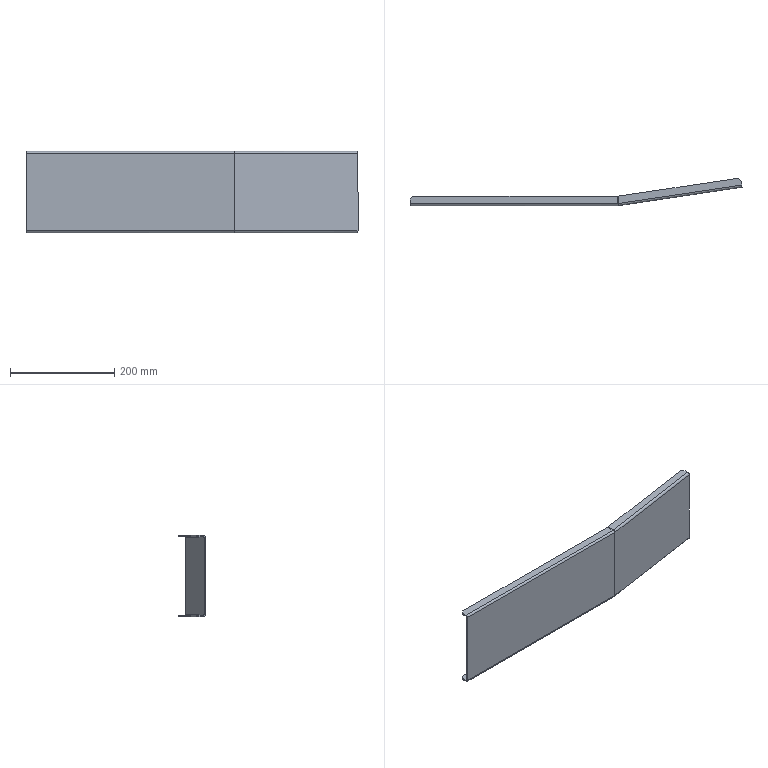Part | SolidWorks | features EdgeFlange 2, Chamfer 1, FlatPattern 1, SMBaseFlange 1, SheetMetal 1 | 1 solid | 54 faces | box 637.587 x 52.537 x 156 mm | volume 352629 mm3 | plane 40 | cylinder 10 | spline 4 | commonest cylinder face diameters 2 x4 8 x4 0.2 x1 6.2 x1